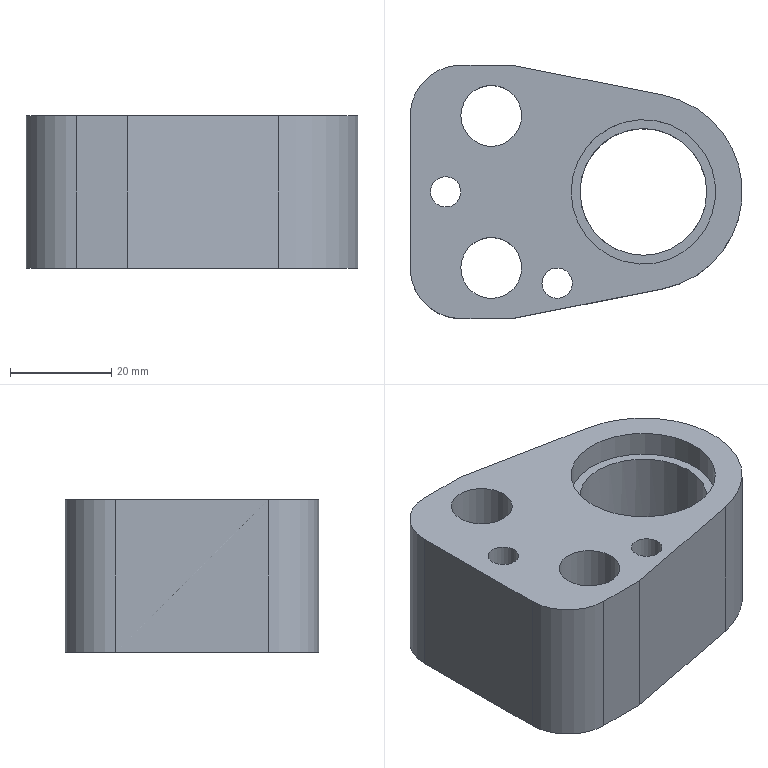Part | NX | features solid 2 | 1 solid | 25 faces | box 65.5 x 50 x 30 mm | volume 54106 mm3 | cylinder 13 | plane 12 | commonest cylinder face diameters 6 x2 8 x2 12 x2 17 x2 20 x2 25 x1
STEP:
#1=CARTESIAN_POINT('',(-603.367,-576.653,71.));
#2=VERTEX_POINT('',#1);
#3=CARTESIAN_POINT('',(-607.367,-576.653,71.));
#4=DIRECTION('',(0.,0.,1.));
#5=DIRECTION('',(1.,0.,0.));
#6=AXIS2_PLACEMENT_3D('',#3,#4,#5);
#7=CIRCLE('',#6,4.);
#8=EDGE_CURVE('',#2,#2,#7,.F.);
#9=ORIENTED_EDGE('',*,*,#8,.F.);
#10=EDGE_LOOP('',(#9));
#11=FACE_BOUND('',#10,.T.);
#12=CARTESIAN_POINT('',(-606.867,-591.653,71.));
#13=VERTEX_POINT('',#12);
#14=CARTESIAN_POINT('',(-598.367,-591.653,71.));
#15=DIRECTION('',(0.,0.,-1.));
#16=DIRECTION('',(-1.,0.,0.));
#17=AXIS2_PLACEMENT_3D('',#14,#15,#16);
#18=CIRCLE('',#17,8.5);
#19=EDGE_CURVE('',#13,#13,#18,.T.);
#20=ORIENTED_EDGE('',*,*,#19,.F.);
#21=EDGE_LOOP('',(#20));
#22=FACE_BOUND('',#21,.T.);
#23=CARTESIAN_POINT('',(-606.867,-561.653,71.));
#24=VERTEX_POINT('',#23);
#25=CARTESIAN_POINT('',(-598.367,-561.653,71.));
#26=DIRECTION('',(0.,0.,-1.));
#27=DIRECTION('',(-1.,0.,0.));
#28=AXIS2_PLACEMENT_3D('',#25,#26,#27);
#29=CIRCLE('',#28,8.5);
#30=EDGE_CURVE('',#24,#24,#29,.T.);
#31=ORIENTED_EDGE('',*,*,#30,.F.);
#32=EDGE_LOOP('',(#31));
#33=FACE_BOUND('',#32,.T.);
#34=CARTESIAN_POINT('',(-555.867,-576.653,71.));
#35=VERTEX_POINT('',#34);
#36=CARTESIAN_POINT('',(-568.367,-576.653,71.));
#37=DIRECTION('',(0.,0.,1.));
#38=DIRECTION('',(1.,0.,0.));
#39=AXIS2_PLACEMENT_3D('',#36,#37,#38);
#40=CIRCLE('',#39,12.5);
#41=EDGE_CURVE('',#35,#35,#40,.T.);
#42=ORIENTED_EDGE('',*,*,#41,.T.);
#43=EDGE_LOOP('',(#42));
#44=FACE_BOUND('',#43,.T.);
#45=CARTESIAN_POINT('',(-564.595,-557.521,71.));
#46=VERTEX_POINT('',#45);
#47=CARTESIAN_POINT('',(-594.367,-551.653,71.));
#48=VERTEX_POINT('',#47);
#49=CARTESIAN_POINT('',(-564.595,-557.521,71.));
#50=DIRECTION('',(-0.9811,0.1934,0.));
#51=VECTOR('',#50,1000.);
#52=LINE('',#49,#51);
#53=EDGE_CURVE('',#46,#48,#52,.T.);
#54=ORIENTED_EDGE('',*,*,#53,.F.);
#55=CARTESIAN_POINT('',(-564.595,-595.785,71.));
#56=VERTEX_POINT('',#55);
#57=CARTESIAN_POINT('',(-568.367,-576.653,71.));
#58=DIRECTION('',(0.,0.,-1.));
#59=DIRECTION('',(-1.,0.,0.));
#60=AXIS2_PLACEMENT_3D('',#57,#58,#59);
#61=CIRCLE('',#60,19.5);
#62=EDGE_CURVE('',#46,#56,#61,.T.);
#63=ORIENTED_EDGE('',*,*,#62,.T.);
#64=CARTESIAN_POINT('',(-594.367,-601.653,71.));
#65=VERTEX_POINT('',#64);
#66=CARTESIAN_POINT('',(-564.595,-595.785,71.));
#67=DIRECTION('',(-0.9811,-0.1934,0.));
#68=VECTOR('',#67,1000.);
#69=LINE('',#66,#68);
#70=EDGE_CURVE('',#56,#65,#69,.T.);
#71=ORIENTED_EDGE('',*,*,#70,.T.);
#72=CARTESIAN_POINT('',(-604.367,-601.653,71.));
#73=VERTEX_POINT('',#72);
#74=CARTESIAN_POINT('',(-594.367,-601.653,71.));
#75=DIRECTION('',(-1.,0.,0.));
#76=VECTOR('',#75,1000.);
#77=LINE('',#74,#76);
#78=EDGE_CURVE('',#65,#73,#77,.T.);
#79=ORIENTED_EDGE('',*,*,#78,.T.);
#80=CARTESIAN_POINT('',(-614.367,-591.653,71.));
#81=VERTEX_POINT('',#80);
#82=CARTESIAN_POINT('',(-604.367,-591.653,71.));
#83=DIRECTION('',(0.,0.,-1.));
#84=DIRECTION('',(-1.,0.,0.));
#85=AXIS2_PLACEMENT_3D('',#82,#83,#84);
#86=CIRCLE('',#85,10.);
#87=EDGE_CURVE('',#73,#81,#86,.T.);
#88=ORIENTED_EDGE('',*,*,#87,.T.);
#89=CARTESIAN_POINT('',(-614.367,-561.653,71.));
#90=VERTEX_POINT('',#89);
#91=CARTESIAN_POINT('',(-614.367,-561.653,71.));
#92=DIRECTION('',(0.,-1.,0.));
#93=VECTOR('',#92,1000.);
#94=LINE('',#91,#93);
#95=EDGE_CURVE('',#90,#81,#94,.T.);
#96=ORIENTED_EDGE('',*,*,#95,.F.);
#97=CARTESIAN_POINT('',(-604.367,-551.653,71.));
#98=VERTEX_POINT('',#97);
#99=CARTESIAN_POINT('',(-604.367,-561.653,71.));
#100=DIRECTION('',(0.,0.,-1.));
#101=DIRECTION('',(-1.,0.,0.));
#102=AXIS2_PLACEMENT_3D('',#99,#100,#101);
#103=CIRCLE('',#102,10.);
#104=EDGE_CURVE('',#90,#98,#103,.T.);
#105=ORIENTED_EDGE('',*,*,#104,.T.);
#106=CARTESIAN_POINT('',(-594.367,-551.653,71.));
#107=DIRECTION('',(-1.,0.,0.));
#108=VECTOR('',#107,1000.);
#109=LINE('',#106,#108);
#110=EDGE_CURVE('',#48,#98,#109,.T.);
#111=ORIENTED_EDGE('',*,*,#110,.F.);
#112=EDGE_LOOP('',(#54,#63,#71,#79,#88,#96,#105,#111));
#113=FACE_BOUND('',#112,.T.);
#114=CARTESIAN_POINT('',(-581.367,-594.653,71.));
#115=VERTEX_POINT('',#114);
#116=CARTESIAN_POINT('',(-585.367,-594.653,71.));
#117=DIRECTION('',(0.,0.,1.));
#118=DIRECTION('',(1.,0.,0.));
#119=AXIS2_PLACEMENT_3D('',#116,#117,#118);
#120=CIRCLE('',#119,4.);
#121=EDGE_CURVE('',#115,#115,#120,.F.);
#122=ORIENTED_EDGE('',*,*,#121,.F.);
#123=EDGE_LOOP('',(#122));
#124=FACE_BOUND('',#123,.T.);
#125=CARTESIAN_POINT('',(-604.367,-561.653,71.));
#126=DIRECTION('',(0.,0.,-1.));
#127=DIRECTION('',(-1.,0.,0.));
#128=AXIS2_PLACEMENT_3D('',#125,#126,#127);
#129=PLANE('',#128);
#130=ADVANCED_FACE('',(#11,#22,#33,#44,#113,#124),#129,.T.);
#131=CARTESIAN_POINT('',(-610.367,-576.653,101.));
#132=VERTEX_POINT('',#131);
#133=CARTESIAN_POINT('',(-607.367,-576.653,101.));
#134=DIRECTION('',(0.,0.,-1.));
#135=DIRECTION('',(-1.,0.,0.));
#136=AXIS2_PLACEMENT_3D('',#133,#134,#135);
#137=CIRCLE('',#136,3.);
#138=EDGE_CURVE('',#132,#132,#137,.T.);
#139=ORIENTED_EDGE('',*,*,#138,.F.);
#140=EDGE_LOOP('',(#139));
#141=FACE_BOUND('',#140,.T.);
#142=CARTESIAN_POINT('',(-610.367,-576.653,91.));
#143=VERTEX_POINT('',#142);
#144=CARTESIAN_POINT('',(-607.367,-576.653,91.));
#145=DIRECTION('',(0.,0.,-1.));
#146=DIRECTION('',(-1.,0.,0.));
#147=AXIS2_PLACEMENT_3D('',#144,#145,#146);
#148=CIRCLE('',#147,3.);
#149=EDGE_CURVE('',#143,#143,#148,.T.);
#150=ORIENTED_EDGE('',*,*,#149,.T.);
#151=EDGE_LOOP('',(#150));
#152=FACE_BOUND('',#151,.T.);
#153=CARTESIAN_POINT('',(-607.367,-576.653,71.));
#154=DIRECTION('',(0.,0.,1.));
#155=DIRECTION('',(1.,0.,0.));
#156=AXIS2_PLACEMENT_3D('',#153,#154,#155);
#157=CYLINDRICAL_SURFACE('',#156,3.);
#158=ADVANCED_FACE('',(#141,#152),#157,.F.);
#159=CARTESIAN_POINT('',(-604.367,-591.653,101.));
#160=VERTEX_POINT('',#159);
#161=CARTESIAN_POINT('',(-598.367,-591.653,101.));
#162=DIRECTION('',(0.,0.,-1.));
#163=DIRECTION('',(-1.,0.,0.));
#164=AXIS2_PLACEMENT_3D('',#161,#162,#163);
#165=CIRCLE('',#164,6.);
#166=EDGE_CURVE('',#160,#160,#165,.T.);
#167=ORIENTED_EDGE('',*,*,#166,.F.);
#168=EDGE_LOOP('',(#167));
#169=FACE_BOUND('',#168,.T.);
#170=CARTESIAN_POINT('',(-604.367,-591.653,83.));
#171=VERTEX_POINT('',#170);
#172=CARTESIAN_POINT('',(-598.367,-591.653,83.));
#173=DIRECTION('',(0.,0.,-1.));
#174=DIRECTION('',(-1.,0.,0.));
#175=AXIS2_PLACEMENT_3D('',#172,#173,#174);
#176=CIRCLE('',#175,6.);
#177=EDGE_CURVE('',#171,#171,#176,.T.);
#178=ORIENTED_EDGE('',*,*,#177,.T.);
#179=EDGE_LOOP('',(#178));
#180=FACE_BOUND('',#179,.T.);
#181=CARTESIAN_POINT('',(-598.367,-591.653,71.));
#182=DIRECTION('',(0.,0.,1.));
#183=DIRECTION('',(1.,0.,0.));
#184=AXIS2_PLACEMENT_3D('',#181,#182,#183);
#185=CYLINDRICAL_SURFACE('',#184,6.);
#186=ADVANCED_FACE('',(#169,#180),#185,.F.);
#187=CARTESIAN_POINT('',(-604.367,-561.653,101.));
#188=VERTEX_POINT('',#187);
#189=CARTESIAN_POINT('',(-598.367,-561.653,101.));
#190=DIRECTION('',(0.,0.,-1.));
#191=DIRECTION('',(-1.,0.,0.));
#192=AXIS2_PLACEMENT_3D('',#189,#190,#191);
#193=CIRCLE('',#192,6.);
#194=EDGE_CURVE('',#188,#188,#193,.T.);
#195=ORIENTED_EDGE('',*,*,#194,.F.);
#196=EDGE_LOOP('',(#195));
#197=FACE_BOUND('',#196,.T.);
#198=CARTESIAN_POINT('',(-604.367,-561.653,83.));
#199=VERTEX_POINT('',#198);
#200=CARTESIAN_POINT('',(-598.367,-561.653,83.));
#201=DIRECTION('',(0.,0.,-1.));
#202=DIRECTION('',(-1.,0.,0.));
#203=AXIS2_PLACEMENT_3D('',#200,#201,#202);
#204=CIRCLE('',#203,6.);
#205=EDGE_CURVE('',#199,#199,#204,.T.);
#206=ORIENTED_EDGE('',*,*,#205,.T.);
#207=EDGE_LOOP('',(#206));
#208=FACE_BOUND('',#207,.T.);
#209=CARTESIAN_POINT('',(-598.367,-561.653,71.));
#210=DIRECTION('',(0.,0.,1.));
#211=DIRECTION('',(1.,0.,0.));
#212=AXIS2_PLACEMENT_3D('',#209,#210,#211);
#213=CYLINDRICAL_SURFACE('',#212,6.);
#214=ADVANCED_FACE('',(#197,#208),#213,.F.);
#215=CARTESIAN_POINT('',(-588.367,-594.653,101.));
#216=VERTEX_POINT('',#215);
#217=CARTESIAN_POINT('',(-585.367,-594.653,101.));
#218=DIRECTION('',(0.,0.,-1.));
#219=DIRECTION('',(-1.,0.,0.));
#220=AXIS2_PLACEMENT_3D('',#217,#218,#219);
#221=CIRCLE('',#220,3.);
#222=EDGE_CURVE('',#216,#216,#221,.T.);
#223=ORIENTED_EDGE('',*,*,#222,.T.);
#224=EDGE_LOOP('',(#223));
#225=FACE_BOUND('',#224,.T.);
#226=ORIENTED_EDGE('',*,*,#166,.T.);
#227=EDGE_LOOP('',(#226));
#228=FACE_BOUND('',#227,.T.);
#229=CARTESIAN_POINT('',(-564.595,-557.521,101.));
#230=VERTEX_POINT('',#229);
#231=CARTESIAN_POINT('',(-594.367,-551.653,101.));
#232=VERTEX_POINT('',#231);
#233=CARTESIAN_POINT('',(-564.595,-557.521,101.));
#234=DIRECTION('',(-0.9811,0.1934,0.));
#235=VECTOR('',#234,1000.);
#236=LINE('',#233,#235);
#237=EDGE_CURVE('',#230,#232,#236,.T.);
#238=ORIENTED_EDGE('',*,*,#237,.T.);
#239=CARTESIAN_POINT('',(-604.367,-551.653,101.));
#240=VERTEX_POINT('',#239);
#241=CARTESIAN_POINT('',(-594.367,-551.653,101.));
#242=DIRECTION('',(-1.,0.,0.));
#243=VECTOR('',#242,1000.);
#244=LINE('',#241,#243);
#245=EDGE_CURVE('',#232,#240,#244,.T.);
#246=ORIENTED_EDGE('',*,*,#245,.T.);
#247=CARTESIAN_POINT('',(-614.367,-561.653,101.));
#248=VERTEX_POINT('',#247);
#249=CARTESIAN_POINT('',(-604.367,-561.653,101.));
#250=DIRECTION('',(0.,0.,-1.));
#251=DIRECTION('',(-1.,0.,0.));
#252=AXIS2_PLACEMENT_3D('',#249,#250,#251);
#253=CIRCLE('',#252,10.);
#254=EDGE_CURVE('',#248,#240,#253,.T.);
#255=ORIENTED_EDGE('',*,*,#254,.F.);
#256=CARTESIAN_POINT('',(-614.367,-591.653,101.));
#257=VERTEX_POINT('',#256);
#258=CARTESIAN_POINT('',(-614.367,-561.653,101.));
#259=DIRECTION('',(0.,-1.,0.));
#260=VECTOR('',#259,1000.);
#261=LINE('',#258,#260);
#262=EDGE_CURVE('',#248,#257,#261,.T.);
#263=ORIENTED_EDGE('',*,*,#262,.T.);
#264=CARTESIAN_POINT('',(-604.367,-601.653,101.));
#265=VERTEX_POINT('',#264);
#266=CARTESIAN_POINT('',(-604.367,-591.653,101.));
#267=DIRECTION('',(0.,0.,-1.));
#268=DIRECTION('',(-1.,0.,0.));
#269=AXIS2_PLACEMENT_3D('',#266,#267,#268);
#270=CIRCLE('',#269,10.);
#271=EDGE_CURVE('',#265,#257,#270,.T.);
#272=ORIENTED_EDGE('',*,*,#271,.F.);
#273=CARTESIAN_POINT('',(-594.367,-601.653,101.));
#274=VERTEX_POINT('',#273);
#275=CARTESIAN_POINT('',(-594.367,-601.653,101.));
#276=DIRECTION('',(-1.,0.,0.));
#277=VECTOR('',#276,1000.);
#278=LINE('',#275,#277);
#279=EDGE_CURVE('',#274,#265,#278,.T.);
#280=ORIENTED_EDGE('',*,*,#279,.F.);
#281=CARTESIAN_POINT('',(-564.595,-595.785,101.));
#282=VERTEX_POINT('',#281);
#283=CARTESIAN_POINT('',(-564.595,-595.785,101.));
#284=DIRECTION('',(-0.9811,-0.1934,0.));
#285=VECTOR('',#284,1000.);
#286=LINE('',#283,#285);
#287=EDGE_CURVE('',#282,#274,#286,.T.);
#288=ORIENTED_EDGE('',*,*,#287,.F.);
#289=CARTESIAN_POINT('',(-568.367,-576.653,101.));
#290=DIRECTION('',(0.,0.,-1.));
#291=DIRECTION('',(-1.,0.,0.));
#292=AXIS2_PLACEMENT_3D('',#289,#290,#291);
#293=CIRCLE('',#292,19.5);
#294=EDGE_CURVE('',#230,#282,#293,.T.);
#295=ORIENTED_EDGE('',*,*,#294,.F.);
#296=EDGE_LOOP('',(#238,#246,#255,#263,#272,#280,#288,#295));
#297=FACE_BOUND('',#296,.T.);
#298=CARTESIAN_POINT('',(-582.617,-576.653,101.));
#299=VERTEX_POINT('',#298);
#300=CARTESIAN_POINT('',(-568.367,-576.653,101.));
#301=DIRECTION('',(0.,0.,-1.));
#302=DIRECTION('',(-1.,0.,0.));
#303=AXIS2_PLACEMENT_3D('',#300,#301,#302);
#304=CIRCLE('',#303,14.25);
#305=EDGE_CURVE('',#299,#299,#304,.T.);
#306=ORIENTED_EDGE('',*,*,#305,.T.);
#307=EDGE_LOOP('',(#306));
#308=FACE_BOUND('',#307,.T.);
#309=ORIENTED_EDGE('',*,*,#194,.T.);
#310=EDGE_LOOP('',(#309));
#311=FACE_BOUND('',#310,.T.);
#312=ORIENTED_EDGE('',*,*,#138,.T.);
#313=EDGE_LOOP('',(#312));
#314=FACE_BOUND('',#313,.T.);
#315=CARTESIAN_POINT('',(-604.367,-561.653,101.));
#316=DIRECTION('',(0.,0.,-1.));
#317=DIRECTION('',(-1.,0.,0.));
#318=AXIS2_PLACEMENT_3D('',#315,#316,#317);
#319=PLANE('',#318);
#320=ADVANCED_FACE('',(#225,#228,#297,#308,#311,#314),#319,.F.);
#321=ORIENTED_EDGE('',*,*,#237,.F.);
#322=CARTESIAN_POINT('',(-564.595,-557.521,71.));
#323=DIRECTION('',(0.,0.,1.));
#324=VECTOR('',#323,1000.);
#325=LINE('',#322,#324);
#326=EDGE_CURVE('',#46,#230,#325,.T.);
#327=ORIENTED_EDGE('',*,*,#326,.F.);
#328=ORIENTED_EDGE('',*,*,#53,.T.);
#329=CARTESIAN_POINT('',(-594.367,-551.653,71.));
#330=DIRECTION('',(0.,0.,1.));
#331=VECTOR('',#330,1000.);
#332=LINE('',#329,#331);
#333=EDGE_CURVE('',#48,#232,#332,.T.);
#334=ORIENTED_EDGE('',*,*,#333,.T.);
#335=EDGE_LOOP('',(#321,#327,#328,#334));
#336=FACE_BOUND('',#335,.T.);
#337=CARTESIAN_POINT('',(-564.595,-557.521,71.));
#338=DIRECTION('',(0.1934,0.9811,0.));
#339=DIRECTION('',(-0.9811,0.1934,0.));
#340=AXIS2_PLACEMENT_3D('',#337,#338,#339);
#341=PLANE('',#340);
#342=ADVANCED_FACE('',(#336),#341,.T.);
#343=ORIENTED_EDGE('',*,*,#245,.F.);
#344=ORIENTED_EDGE('',*,*,#333,.F.);
#345=ORIENTED_EDGE('',*,*,#110,.T.);
#346=CARTESIAN_POINT('',(-604.367,-551.653,71.));
#347=DIRECTION('',(0.,0.,1.));
#348=VECTOR('',#347,1000.);
#349=LINE('',#346,#348);
#350=EDGE_CURVE('',#98,#240,#349,.T.);
#351=ORIENTED_EDGE('',*,*,#350,.T.);
#352=EDGE_LOOP('',(#343,#344,#345,#351));
#353=FACE_BOUND('',#352,.T.);
#354=CARTESIAN_POINT('',(-594.367,-551.653,71.));
#355=DIRECTION('',(0.,1.,0.));
#356=DIRECTION('',(0.,0.,1.));
#357=AXIS2_PLACEMENT_3D('',#354,#355,#356);
#358=PLANE('',#357);
#359=ADVANCED_FACE('',(#353),#358,.T.);
#360=ORIENTED_EDGE('',*,*,#254,.T.);
#361=ORIENTED_EDGE('',*,*,#350,.F.);
#362=ORIENTED_EDGE('',*,*,#104,.F.);
#363=CARTESIAN_POINT('',(-614.367,-561.653,71.));
#364=DIRECTION('',(0.,0.,1.));
#365=VECTOR('',#364,1000.);
#366=LINE('',#363,#365);
#367=EDGE_CURVE('',#90,#248,#366,.T.);
#368=ORIENTED_EDGE('',*,*,#367,.T.);
#369=EDGE_LOOP('',(#360,#361,#362,#368));
#370=FACE_BOUND('',#369,.T.);
#371=CARTESIAN_POINT('',(-604.367,-561.653,71.));
#372=DIRECTION('',(0.,0.,1.));
#373=DIRECTION('',(1.,0.,0.));
#374=AXIS2_PLACEMENT_3D('',#371,#372,#373);
#375=CYLINDRICAL_SURFACE('',#374,10.);
#376=ADVANCED_FACE('',(#370),#375,.T.);
#377=ORIENTED_EDGE('',*,*,#262,.F.);
#378=ORIENTED_EDGE('',*,*,#367,.F.);
#379=ORIENTED_EDGE('',*,*,#95,.T.);
#380=CARTESIAN_POINT('',(-614.367,-591.653,71.));
#381=DIRECTION('',(0.,0.,1.));
#382=VECTOR('',#381,1000.);
#383=LINE('',#380,#382);
#384=EDGE_CURVE('',#81,#257,#383,.T.);
#385=ORIENTED_EDGE('',*,*,#384,.T.);
#386=EDGE_LOOP('',(#377,#378,#379,#385));
#387=FACE_BOUND('',#386,.T.);
#388=CARTESIAN_POINT('',(-614.367,-561.653,71.));
#389=DIRECTION('',(-1.,0.,0.));
#390=DIRECTION('',(0.,-1.,0.));
#391=AXIS2_PLACEMENT_3D('',#388,#389,#390);
#392=PLANE('',#391);
#393=ADVANCED_FACE('',(#387),#392,.T.);
#394=ORIENTED_EDGE('',*,*,#271,.T.);
#395=ORIENTED_EDGE('',*,*,#384,.F.);
#396=ORIENTED_EDGE('',*,*,#87,.F.);
#397=CARTESIAN_POINT('',(-604.367,-601.653,71.));
#398=DIRECTION('',(0.,0.,1.));
#399=VECTOR('',#398,1000.);
#400=LINE('',#397,#399);
#401=EDGE_CURVE('',#73,#265,#400,.T.);
#402=ORIENTED_EDGE('',*,*,#401,.T.);
#403=EDGE_LOOP('',(#394,#395,#396,#402));
#404=FACE_BOUND('',#403,.T.);
#405=CARTESIAN_POINT('',(-604.367,-591.653,71.));
#406=DIRECTION('',(0.,0.,1.));
#407=DIRECTION('',(1.,0.,0.));
#408=AXIS2_PLACEMENT_3D('',#405,#406,#407);
#409=CYLINDRICAL_SURFACE('',#408,10.);
#410=ADVANCED_FACE('',(#404),#409,.T.);
#411=ORIENTED_EDGE('',*,*,#279,.T.);
#412=ORIENTED_EDGE('',*,*,#401,.F.);
#413=ORIENTED_EDGE('',*,*,#78,.F.);
#414=CARTESIAN_POINT('',(-594.367,-601.653,71.));
#415=DIRECTION('',(0.,0.,1.));
#416=VECTOR('',#415,1000.);
#417=LINE('',#414,#416);
#418=EDGE_CURVE('',#65,#274,#417,.T.);
#419=ORIENTED_EDGE('',*,*,#418,.T.);
#420=EDGE_LOOP('',(#411,#412,#413,#419));
#421=FACE_BOUND('',#420,.T.);
#422=CARTESIAN_POINT('',(-594.367,-601.653,71.));
#423=DIRECTION('',(0.,1.,0.));
#424=DIRECTION('',(-1.,0.,0.));
#425=AXIS2_PLACEMENT_3D('',#422,#423,#424);
#426=PLANE('',#425);
#427=ADVANCED_FACE('',(#421),#426,.F.);
#428=ORIENTED_EDGE('',*,*,#287,.T.);
#429=ORIENTED_EDGE('',*,*,#418,.F.);
#430=ORIENTED_EDGE('',*,*,#70,.F.);
#431=CARTESIAN_POINT('',(-564.595,-595.785,71.));
#432=DIRECTION('',(0.,0.,1.));
#433=VECTOR('',#432,1000.);
#434=LINE('',#431,#433);
#435=EDGE_CURVE('',#56,#282,#434,.T.);
#436=ORIENTED_EDGE('',*,*,#435,.T.);
#437=EDGE_LOOP('',(#428,#429,#430,#436));
#438=FACE_BOUND('',#437,.T.);
#439=CARTESIAN_POINT('',(-564.595,-595.785,71.));
#440=DIRECTION('',(-0.1934,0.9811,0.));
#441=DIRECTION('',(-0.9811,-0.1934,0.));
#442=AXIS2_PLACEMENT_3D('',#439,#440,#441);
#443=PLANE('',#442);
#444=ADVANCED_FACE('',(#438),#443,.F.);
#445=ORIENTED_EDGE('',*,*,#294,.T.);
#446=ORIENTED_EDGE('',*,*,#435,.F.);
#447=ORIENTED_EDGE('',*,*,#62,.F.);
#448=ORIENTED_EDGE('',*,*,#326,.T.);
#449=EDGE_LOOP('',(#445,#446,#447,#448));
#450=FACE_BOUND('',#449,.T.);
#451=CARTESIAN_POINT('',(-568.367,-576.653,71.));
#452=DIRECTION('',(0.,0.,1.));
#453=DIRECTION('',(1.,0.,0.));
#454=AXIS2_PLACEMENT_3D('',#451,#452,#453);
#455=CYLINDRICAL_SURFACE('',#454,19.5);
#456=ADVANCED_FACE('',(#450),#455,.T.);
#457=CARTESIAN_POINT('',(-580.867,-576.653,96.));
#458=VERTEX_POINT('',#457);
#459=CARTESIAN_POINT('',(-568.367,-576.653,96.));
#460=DIRECTION('',(0.,0.,-1.));
#461=DIRECTION('',(-1.,0.,0.));
#462=AXIS2_PLACEMENT_3D('',#459,#460,#461);
#463=CIRCLE('',#462,12.5);
#464=EDGE_CURVE('',#458,#458,#463,.F.);
#465=ORIENTED_EDGE('',*,*,#464,.T.);
#466=EDGE_LOOP('',(#465));
#467=FACE_BOUND('',#466,.T.);
#468=ORIENTED_EDGE('',*,*,#41,.F.);
#469=EDGE_LOOP('',(#468));
#470=FACE_BOUND('',#469,.T.);
#471=CARTESIAN_POINT('',(-568.367,-576.653,71.));
#472=DIRECTION('',(0.,0.,1.));
#473=DIRECTION('',(1.,0.,0.));
#474=AXIS2_PLACEMENT_3D('',#471,#472,#473);
#475=CYLINDRICAL_SURFACE('',#474,12.5);
#476=ADVANCED_FACE('',(#467,#470),#475,.F.);
#477=CARTESIAN_POINT('',(-582.617,-576.653,96.));
#478=VERTEX_POINT('',#477);
#479=CARTESIAN_POINT('',(-568.367,-576.653,96.));
#480=DIRECTION('',(0.,0.,-1.));
#481=DIRECTION('',(-1.,0.,0.));
#482=AXIS2_PLACEMENT_3D('',#479,#480,#481);
#483=CIRCLE('',#482,14.25);
#484=EDGE_CURVE('',#478,#478,#483,.T.);
#485=ORIENTED_EDGE('',*,*,#484,.F.);
#486=EDGE_LOOP('',(#485));
#487=FACE_BOUND('',#486,.T.);
#488=ORIENTED_EDGE('',*,*,#464,.F.);
#489=EDGE_LOOP('',(#488));
#490=FACE_BOUND('',#489,.T.);
#491=CARTESIAN_POINT('',(-568.367,-576.653,96.));
#492=DIRECTION('',(0.,0.,-1.));
#493=DIRECTION('',(-1.,0.,0.));
#494=AXIS2_PLACEMENT_3D('',#491,#492,#493);
#495=PLANE('',#494);
#496=ADVANCED_FACE('',(#487,#490),#495,.F.);
#497=ORIENTED_EDGE('',*,*,#484,.T.);
#498=EDGE_LOOP('',(#497));
#499=FACE_BOUND('',#498,.T.);
#500=ORIENTED_EDGE('',*,*,#305,.F.);
#501=EDGE_LOOP('',(#500));
#502=FACE_BOUND('',#501,.T.);
#503=CARTESIAN_POINT('',(-568.367,-576.653,96.));
#504=DIRECTION('',(0.,0.,1.));
#505=DIRECTION('',(1.,0.,0.));
#506=AXIS2_PLACEMENT_3D('',#503,#504,#505);
#507=CYLINDRICAL_SURFACE('',#506,14.25);
#508=ADVANCED_FACE('',(#499,#502),#507,.F.);
#509=CARTESIAN_POINT('',(-588.367,-594.653,91.));
#510=VERTEX_POINT('',#509);
#511=CARTESIAN_POINT('',(-585.367,-594.653,91.));
#512=DIRECTION('',(0.,0.,-1.));
#513=DIRECTION('',(-1.,0.,0.));
#514=AXIS2_PLACEMENT_3D('',#511,#512,#513);
#515=CIRCLE('',#514,3.);
#516=EDGE_CURVE('',#510,#510,#515,.T.);
#517=ORIENTED_EDGE('',*,*,#516,.T.);
#518=EDGE_LOOP('',(#517));
#519=FACE_BOUND('',#518,.T.);
#520=ORIENTED_EDGE('',*,*,#222,.F.);
#521=EDGE_LOOP('',(#520));
#522=FACE_BOUND('',#521,.T.);
#523=CARTESIAN_POINT('',(-585.367,-594.653,71.));
#524=DIRECTION('',(0.,0.,1.));
#525=DIRECTION('',(1.,0.,0.));
#526=AXIS2_PLACEMENT_3D('',#523,#524,#525);
#527=CYLINDRICAL_SURFACE('',#526,3.);
#528=ADVANCED_FACE('',(#519,#522),#527,.F.);
#529=CARTESIAN_POINT('',(-606.867,-561.653,83.));
#530=VERTEX_POINT('',#529);
#531=CARTESIAN_POINT('',(-598.367,-561.653,83.));
#532=DIRECTION('',(0.,0.,-1.));
#533=DIRECTION('',(-1.,0.,0.));
#534=AXIS2_PLACEMENT_3D('',#531,#532,#533);
#535=CIRCLE('',#534,8.5);
#536=EDGE_CURVE('',#530,#530,#535,.T.);
#537=ORIENTED_EDGE('',*,*,#536,.F.);
#538=EDGE_LOOP('',(#537));
#539=FACE_BOUND('',#538,.T.);
#540=ORIENTED_EDGE('',*,*,#30,.T.);
#541=EDGE_LOOP('',(#540));
#542=FACE_BOUND('',#541,.T.);
#543=CARTESIAN_POINT('',(-598.367,-561.653,83.));
#544=DIRECTION('',(0.,0.,-1.));
#545=DIRECTION('',(-1.,0.,0.));
#546=AXIS2_PLACEMENT_3D('',#543,#544,#545);
#547=CYLINDRICAL_SURFACE('',#546,8.5);
#548=ADVANCED_FACE('',(#539,#542),#547,.F.);
#549=ORIENTED_EDGE('',*,*,#205,.F.);
#550=EDGE_LOOP('',(#549));
#551=FACE_BOUND('',#550,.T.);
#552=ORIENTED_EDGE('',*,*,#536,.T.);
#553=EDGE_LOOP('',(#552));
#554=FACE_BOUND('',#553,.T.);
#555=CARTESIAN_POINT('',(-598.367,-561.653,83.));
#556=DIRECTION('',(0.,0.,-1.));
#557=DIRECTION('',(-1.,0.,0.));
#558=AXIS2_PLACEMENT_3D('',#555,#556,#557);
#559=PLANE('',#558);
#560=ADVANCED_FACE('',(#551,#554),#559,.T.);
#561=CARTESIAN_POINT('',(-606.867,-591.653,83.));
#562=VERTEX_POINT('',#561);
#563=CARTESIAN_POINT('',(-598.367,-591.653,83.));
#564=DIRECTION('',(0.,0.,-1.));
#565=DIRECTION('',(-1.,0.,0.));
#566=AXIS2_PLACEMENT_3D('',#563,#564,#565);
#567=CIRCLE('',#566,8.5);
#568=EDGE_CURVE('',#562,#562,#567,.T.);
#569=ORIENTED_EDGE('',*,*,#568,.F.);
#570=EDGE_LOOP('',(#569));
#571=FACE_BOUND('',#570,.T.);
#572=ORIENTED_EDGE('',*,*,#19,.T.);
#573=EDGE_LOOP('',(#572));
#574=FACE_BOUND('',#573,.T.);
#575=CARTESIAN_POINT('',(-598.367,-591.653,83.));
#576=DIRECTION('',(0.,0.,-1.));
#577=DIRECTION('',(-1.,0.,0.));
#578=AXIS2_PLACEMENT_3D('',#575,#576,#577);
#579=CYLINDRICAL_SURFACE('',#578,8.5);
#580=ADVANCED_FACE('',(#571,#574),#579,.F.);
#581=ORIENTED_EDGE('',*,*,#177,.F.);
#582=EDGE_LOOP('',(#581));
#583=FACE_BOUND('',#582,.T.);
#584=ORIENTED_EDGE('',*,*,#568,.T.);
#585=EDGE_LOOP('',(#584));
#586=FACE_BOUND('',#585,.T.);
#587=CARTESIAN_POINT('',(-598.367,-591.653,83.));
#588=DIRECTION('',(0.,0.,-1.));
#589=DIRECTION('',(-1.,0.,0.));
#590=AXIS2_PLACEMENT_3D('',#587,#588,#589);
#591=PLANE('',#590);
#592=ADVANCED_FACE('',(#583,#586),#591,.T.);
#593=ORIENTED_EDGE('',*,*,#149,.F.);
#594=EDGE_LOOP('',(#593));
#595=FACE_BOUND('',#594,.T.);
#596=CARTESIAN_POINT('',(-603.367,-576.653,91.));
#597=VERTEX_POINT('',#596);
#598=CARTESIAN_POINT('',(-607.367,-576.653,91.));
#599=DIRECTION('',(0.,0.,1.));
#600=DIRECTION('',(1.,0.,0.));
#601=AXIS2_PLACEMENT_3D('',#598,#599,#600);
#602=CIRCLE('',#601,4.);
#603=EDGE_CURVE('',#597,#597,#602,.F.);
#604=ORIENTED_EDGE('',*,*,#603,.T.);
#605=EDGE_LOOP('',(#604));
#606=FACE_BOUND('',#605,.T.);
#607=CARTESIAN_POINT('',(-607.367,-576.653,91.));
#608=DIRECTION('',(0.,0.,1.));
#609=DIRECTION('',(1.,0.,0.));
#610=AXIS2_PLACEMENT_3D('',#607,#608,#609);
#611=PLANE('',#610);
#612=ADVANCED_FACE('',(#595,#606),#611,.F.);
#613=ORIENTED_EDGE('',*,*,#603,.F.);
#614=EDGE_LOOP('',(#613));
#615=FACE_BOUND('',#614,.T.);
#616=ORIENTED_EDGE('',*,*,#8,.T.);
#617=EDGE_LOOP('',(#616));
#618=FACE_BOUND('',#617,.T.);
#619=CARTESIAN_POINT('',(-607.367,-576.653,71.));
#620=DIRECTION('',(0.,0.,1.));
#621=DIRECTION('',(1.,0.,0.));
#622=AXIS2_PLACEMENT_3D('',#619,#620,#621);
#623=CYLINDRICAL_SURFACE('',#622,4.);
#624=ADVANCED_FACE('',(#615,#618),#623,.F.);
#625=ORIENTED_EDGE('',*,*,#516,.F.);
#626=EDGE_LOOP('',(#625));
#627=FACE_BOUND('',#626,.T.);
#628=CARTESIAN_POINT('',(-581.367,-594.653,91.));
#629=VERTEX_POINT('',#628);
#630=CARTESIAN_POINT('',(-585.367,-594.653,91.));
#631=DIRECTION('',(0.,0.,1.));
#632=DIRECTION('',(1.,0.,0.));
#633=AXIS2_PLACEMENT_3D('',#630,#631,#632);
#634=CIRCLE('',#633,4.);
#635=EDGE_CURVE('',#629,#629,#634,.F.);
#636=ORIENTED_EDGE('',*,*,#635,.T.);
#637=EDGE_LOOP('',(#636));
#638=FACE_BOUND('',#637,.T.);
#639=CARTESIAN_POINT('',(-585.367,-594.653,91.));
#640=DIRECTION('',(0.,0.,1.));
#641=DIRECTION('',(1.,0.,0.));
#642=AXIS2_PLACEMENT_3D('',#639,#640,#641);
#643=PLANE('',#642);
#644=ADVANCED_FACE('',(#627,#638),#643,.F.);
#645=ORIENTED_EDGE('',*,*,#635,.F.);
#646=EDGE_LOOP('',(#645));
#647=FACE_BOUND('',#646,.T.);
#648=ORIENTED_EDGE('',*,*,#121,.T.);
#649=EDGE_LOOP('',(#648));
#650=FACE_BOUND('',#649,.T.);
#651=CARTESIAN_POINT('',(-585.367,-594.653,71.));
#652=DIRECTION('',(0.,0.,1.));
#653=DIRECTION('',(1.,0.,0.));
#654=AXIS2_PLACEMENT_3D('',#651,#652,#653);
#655=CYLINDRICAL_SURFACE('',#654,4.);
#656=ADVANCED_FACE('',(#647,#650),#655,.F.);
#657=CLOSED_SHELL('',(#130,#158,#186,#214,#320,#342,#359,#376,#393,#410,#427,#444,#456,#476,#496,#508,#528,#548,#560,#580,#592,#612,#624,#644,#656));
#658=MANIFOLD_SOLID_BREP('',#657);
#659=(LENGTH_UNIT()NAMED_UNIT(*)SI_UNIT(.MILLI.,.METRE.));
#660=UNCERTAINTY_MEASURE_WITH_UNIT(LENGTH_MEASURE(0.00001),#659,'','');
#661=(NAMED_UNIT(*)PLANE_ANGLE_UNIT()SI_UNIT($,.RADIAN.));
#662=(NAMED_UNIT(*)SI_UNIT($,.STERADIAN.)SOLID_ANGLE_UNIT());
#663=(GEOMETRIC_REPRESENTATION_CONTEXT(3)GLOBAL_UNCERTAINTY_ASSIGNED_CONTEXT((#660))GLOBAL_UNIT_ASSIGNED_CONTEXT((#659,#661,#662))REPRESENTATION_CONTEXT('',''));
#664=ADVANCED_BREP_SHAPE_REPRESENTATION('',(#658),#663);